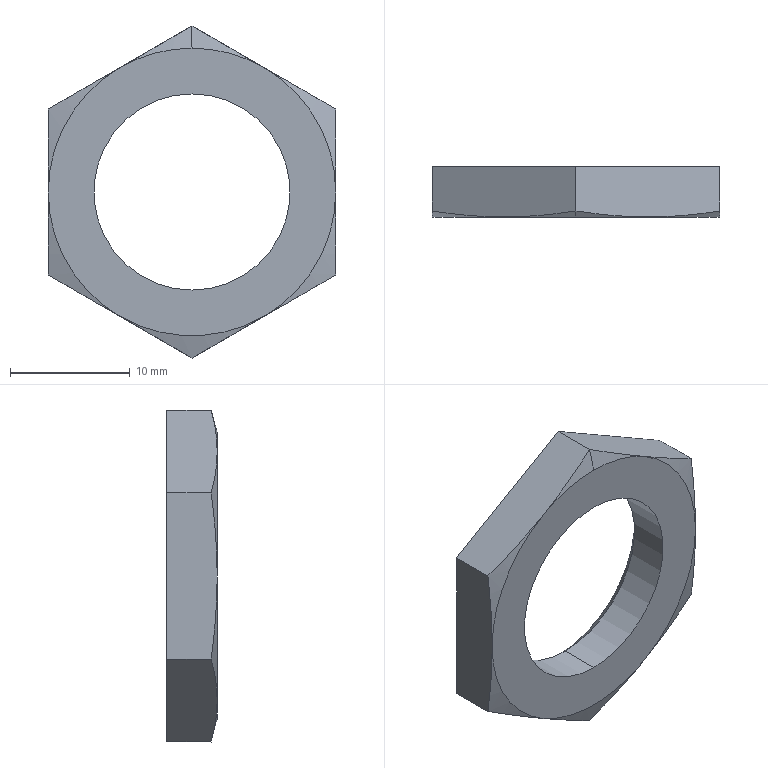Part | SolidWorks | features BaseBody 1 | 1 solid | 19 faces | box 24 x 4.2 x 27.713 mm | volume 1186 mm3 | cone 9 | plane 8 | cylinder 2 | commonest cylinder face diameters 16.376 x2
STEP:
#1=CARTESIAN_POINT('',(137.047,1614.26,-1167.188));
#2=VERTEX_POINT('',#1);
#3=CARTESIAN_POINT('',(137.047,1614.26,-1150.812));
#4=VERTEX_POINT('',#3);
#5=CARTESIAN_POINT('',(137.047,1614.26,-1159.));
#6=DIRECTION('',(0.,1.,0.));
#7=DIRECTION('',(0.,0.,-1.));
#8=AXIS2_PLACEMENT_3D('',#5,#6,#7);
#9=CIRCLE('',#8,8.188);
#10=EDGE_CURVE('',#2,#4,#9,.T.);
#11=ORIENTED_EDGE('',*,*,#10,.F.);
#12=CARTESIAN_POINT('',(137.047,1615.079,-1168.007));
#13=VERTEX_POINT('',#12);
#14=CARTESIAN_POINT('',(137.047,1615.079,-1168.007));
#15=DIRECTION('',(0.,0.7071,-0.7071));
#16=VECTOR('',#15,1000.);
#17=LINE('',#14,#16);
#18=EDGE_CURVE('',#2,#13,#17,.T.);
#19=ORIENTED_EDGE('',*,*,#18,.T.);
#20=CARTESIAN_POINT('',(137.047,1615.079,-1149.993));
#21=VERTEX_POINT('',#20);
#22=CARTESIAN_POINT('',(137.047,1615.079,-1159.));
#23=DIRECTION('',(0.,-1.,0.));
#24=DIRECTION('',(0.,0.,1.));
#25=AXIS2_PLACEMENT_3D('',#22,#23,#24);
#26=CIRCLE('',#25,9.007);
#27=EDGE_CURVE('',#21,#13,#26,.T.);
#28=ORIENTED_EDGE('',*,*,#27,.F.);
#29=CARTESIAN_POINT('',(137.047,1615.079,-1149.993));
#30=DIRECTION('',(0.,0.7071,0.7071));
#31=VECTOR('',#30,1000.);
#32=LINE('',#29,#31);
#33=EDGE_CURVE('',#4,#21,#32,.T.);
#34=ORIENTED_EDGE('',*,*,#33,.F.);
#35=EDGE_LOOP('',(#11,#19,#28,#34));
#36=FACE_OUTER_BOUND('',#35,.T.);
#37=CARTESIAN_POINT('',(137.047,1615.079,-1159.));
#38=DIRECTION('',(0.,1.,0.));
#39=DIRECTION('',(0.,0.,1.));
#40=AXIS2_PLACEMENT_3D('',#37,#38,#39);
#41=CONICAL_SURFACE('',#40,9.007,0.7854);
#42=ADVANCED_FACE('',(#36),#41,.F.);
#43=CARTESIAN_POINT('',(137.047,1610.879,-1167.188));
#44=VERTEX_POINT('',#43);
#45=CARTESIAN_POINT('',(137.047,1610.879,-1150.812));
#46=VERTEX_POINT('',#45);
#47=CARTESIAN_POINT('',(137.047,1610.879,-1159.));
#48=DIRECTION('',(0.,1.,0.));
#49=DIRECTION('',(0.,0.,1.));
#50=AXIS2_PLACEMENT_3D('',#47,#48,#49);
#51=CIRCLE('',#50,8.188);
#52=EDGE_CURVE('',#44,#46,#51,.T.);
#53=ORIENTED_EDGE('',*,*,#52,.F.);
#54=CARTESIAN_POINT('',(137.047,1610.879,-1167.188));
#55=DIRECTION('',(0.,1.,0.));
#56=VECTOR('',#55,1000.);
#57=LINE('',#54,#56);
#58=EDGE_CURVE('',#44,#2,#57,.T.);
#59=ORIENTED_EDGE('',*,*,#58,.T.);
#60=ORIENTED_EDGE('',*,*,#10,.T.);
#61=CARTESIAN_POINT('',(137.047,1610.879,-1150.812));
#62=DIRECTION('',(0.,1.,0.));
#63=VECTOR('',#62,1000.);
#64=LINE('',#61,#63);
#65=EDGE_CURVE('',#46,#4,#64,.T.);
#66=ORIENTED_EDGE('',*,*,#65,.F.);
#67=EDGE_LOOP('',(#53,#59,#60,#66));
#68=FACE_OUTER_BOUND('',#67,.T.);
#69=CARTESIAN_POINT('',(137.047,1610.879,-1159.));
#70=DIRECTION('',(0.,1.,0.));
#71=DIRECTION('',(0.,0.,1.));
#72=AXIS2_PLACEMENT_3D('',#69,#70,#71);
#73=CYLINDRICAL_SURFACE('',#72,8.188);
#74=ADVANCED_FACE('',(#68),#73,.F.);
#75=CARTESIAN_POINT('',(131.047,1610.879,-1148.608));
#76=VERTEX_POINT('',#75);
#77=CARTESIAN_POINT('',(137.047,1610.879,-1147.));
#78=VERTEX_POINT('',#77);
#79=CARTESIAN_POINT('',(137.047,1610.879,-1159.));
#80=DIRECTION('',(0.,1.,0.));
#81=DIRECTION('',(0.,0.,1.));
#82=AXIS2_PLACEMENT_3D('',#79,#80,#81);
#83=CIRCLE('',#82,12.);
#84=EDGE_CURVE('',#76,#78,#83,.T.);
#85=ORIENTED_EDGE('',*,*,#84,.T.);
#86=CARTESIAN_POINT('',(137.047,1611.376,-1145.144));
#87=VERTEX_POINT('',#86);
#88=CARTESIAN_POINT('',(137.047,1611.379,-1145.132));
#89=DIRECTION('',(0.,0.2588,0.9659));
#90=VECTOR('',#89,1000.);
#91=LINE('',#88,#90);
#92=EDGE_CURVE('',#78,#87,#91,.T.);
#93=ORIENTED_EDGE('',*,*,#92,.T.);
#94=CARTESIAN_POINT('',(131.047,1610.879,-1148.608));
#95=CARTESIAN_POINT('',(132.052,1610.879,-1148.027));
#96=CARTESIAN_POINT('',(133.054,1610.925,-1147.449));
#97=CARTESIAN_POINT('',(135.054,1611.097,-1146.294));
#98=CARTESIAN_POINT('',(136.051,1611.222,-1145.718));
#99=CARTESIAN_POINT('',(137.047,1611.376,-1145.144));
#100=B_SPLINE_CURVE_WITH_KNOTS('',3,(#94,#95,#96,#97,#98,#99),.UNSPECIFIED.,.F.,.F.,(4,2,4),(0.,0.003473,0.006946),.UNSPECIFIED.);
#101=EDGE_CURVE('',#76,#87,#100,.T.);
#102=ORIENTED_EDGE('',*,*,#101,.F.);
#103=EDGE_LOOP('',(#85,#93,#102));
#104=FACE_OUTER_BOUND('',#103,.T.);
#105=CARTESIAN_POINT('',(137.047,1611.379,-1159.));
#106=DIRECTION('',(0.,1.,0.));
#107=DIRECTION('',(0.,0.,1.));
#108=AXIS2_PLACEMENT_3D('',#105,#106,#107);
#109=CONICAL_SURFACE('',#108,13.868,1.309);
#110=ADVANCED_FACE('',(#104),#109,.T.);
#111=ORIENTED_EDGE('',*,*,#27,.T.);
#112=CARTESIAN_POINT('',(137.047,1615.079,-1159.));
#113=DIRECTION('',(0.,-1.,0.));
#114=DIRECTION('',(0.,0.,1.));
#115=AXIS2_PLACEMENT_3D('',#112,#113,#114);
#116=CIRCLE('',#115,9.007);
#117=EDGE_CURVE('',#13,#21,#116,.T.);
#118=ORIENTED_EDGE('',*,*,#117,.T.);
#119=EDGE_LOOP('',(#111,#118));
#120=FACE_BOUND('',#119,.T.);
#121=CARTESIAN_POINT('',(137.047,1615.079,-1145.144));
#122=VERTEX_POINT('',#121);
#123=CARTESIAN_POINT('',(149.047,1615.079,-1152.072));
#124=VERTEX_POINT('',#123);
#125=CARTESIAN_POINT('',(137.047,1615.079,-1145.144));
#126=DIRECTION('',(0.866,0.,-0.5));
#127=VECTOR('',#126,1000.);
#128=LINE('',#125,#127);
#129=EDGE_CURVE('',#122,#124,#128,.T.);
#130=ORIENTED_EDGE('',*,*,#129,.T.);
#131=CARTESIAN_POINT('',(149.047,1615.079,-1165.928));
#132=VERTEX_POINT('',#131);
#133=CARTESIAN_POINT('',(149.047,1615.079,-1165.928));
#134=DIRECTION('',(0.,0.,-1.));
#135=VECTOR('',#134,1000.);
#136=LINE('',#133,#135);
#137=EDGE_CURVE('',#124,#132,#136,.T.);
#138=ORIENTED_EDGE('',*,*,#137,.T.);
#139=CARTESIAN_POINT('',(137.047,1615.079,-1172.856));
#140=VERTEX_POINT('',#139);
#141=CARTESIAN_POINT('',(149.047,1615.079,-1165.928));
#142=DIRECTION('',(-0.866,0.,-0.5));
#143=VECTOR('',#142,1000.);
#144=LINE('',#141,#143);
#145=EDGE_CURVE('',#132,#140,#144,.T.);
#146=ORIENTED_EDGE('',*,*,#145,.T.);
#147=CARTESIAN_POINT('',(125.047,1615.079,-1165.928));
#148=VERTEX_POINT('',#147);
#149=CARTESIAN_POINT('',(137.047,1615.079,-1172.856));
#150=DIRECTION('',(-0.866,0.,0.5));
#151=VECTOR('',#150,1000.);
#152=LINE('',#149,#151);
#153=EDGE_CURVE('',#140,#148,#152,.T.);
#154=ORIENTED_EDGE('',*,*,#153,.T.);
#155=CARTESIAN_POINT('',(125.047,1615.079,-1152.072));
#156=VERTEX_POINT('',#155);
#157=CARTESIAN_POINT('',(125.047,1615.079,-1165.928));
#158=DIRECTION('',(0.,0.,1.));
#159=VECTOR('',#158,1000.);
#160=LINE('',#157,#159);
#161=EDGE_CURVE('',#148,#156,#160,.T.);
#162=ORIENTED_EDGE('',*,*,#161,.T.);
#163=CARTESIAN_POINT('',(125.047,1615.079,-1152.072));
#164=DIRECTION('',(0.866,0.,0.5));
#165=VECTOR('',#164,1000.);
#166=LINE('',#163,#165);
#167=EDGE_CURVE('',#156,#122,#166,.T.);
#168=ORIENTED_EDGE('',*,*,#167,.T.);
#169=EDGE_LOOP('',(#130,#138,#146,#154,#162,#168));
#170=FACE_OUTER_BOUND('',#169,.T.);
#171=CARTESIAN_POINT('',(149.047,1615.079,-1165.928));
#172=DIRECTION('',(0.,1.,0.));
#173=DIRECTION('',(0.,0.,1.));
#174=AXIS2_PLACEMENT_3D('',#171,#172,#173);
#175=PLANE('',#174);
#176=ADVANCED_FACE('',(#120,#170),#175,.T.);
#177=ORIENTED_EDGE('',*,*,#18,.F.);
#178=CARTESIAN_POINT('',(137.047,1614.26,-1159.));
#179=DIRECTION('',(0.,1.,0.));
#180=DIRECTION('',(0.,0.,-1.));
#181=AXIS2_PLACEMENT_3D('',#178,#179,#180);
#182=CIRCLE('',#181,8.188);
#183=EDGE_CURVE('',#4,#2,#182,.T.);
#184=ORIENTED_EDGE('',*,*,#183,.F.);
#185=ORIENTED_EDGE('',*,*,#33,.T.);
#186=ORIENTED_EDGE('',*,*,#117,.F.);
#187=EDGE_LOOP('',(#177,#184,#185,#186));
#188=FACE_OUTER_BOUND('',#187,.T.);
#189=CARTESIAN_POINT('',(137.047,1615.079,-1159.));
#190=DIRECTION('',(0.,1.,0.));
#191=DIRECTION('',(0.,0.,1.));
#192=AXIS2_PLACEMENT_3D('',#189,#190,#191);
#193=CONICAL_SURFACE('',#192,9.007,0.7854);
#194=ADVANCED_FACE('',(#188),#193,.F.);
#195=CARTESIAN_POINT('',(149.047,1611.376,-1152.072));
#196=VERTEX_POINT('',#195);
#197=CARTESIAN_POINT('',(149.047,1610.879,-1159.));
#198=VERTEX_POINT('',#197);
#199=CARTESIAN_POINT('',(149.047,1611.376,-1152.072));
#200=CARTESIAN_POINT('',(149.047,1611.222,-1153.221));
#201=CARTESIAN_POINT('',(149.047,1611.097,-1154.373));
#202=CARTESIAN_POINT('',(149.047,1610.925,-1156.682));
#203=CARTESIAN_POINT('',(149.047,1610.879,-1157.839));
#204=CARTESIAN_POINT('',(149.047,1610.879,-1159.));
#205=B_SPLINE_CURVE_WITH_KNOTS('',3,(#199,#200,#201,#202,#203,#204),.UNSPECIFIED.,.F.,.F.,(4,2,4),(0.,0.003473,0.006946),.UNSPECIFIED.);
#206=EDGE_CURVE('',#196,#198,#205,.T.);
#207=ORIENTED_EDGE('',*,*,#206,.T.);
#208=CARTESIAN_POINT('',(149.047,1611.376,-1165.928));
#209=VERTEX_POINT('',#208);
#210=CARTESIAN_POINT('',(149.047,1610.879,-1159.));
#211=CARTESIAN_POINT('',(149.047,1610.879,-1160.161));
#212=CARTESIAN_POINT('',(149.047,1610.925,-1161.318));
#213=CARTESIAN_POINT('',(149.047,1611.097,-1163.627));
#214=CARTESIAN_POINT('',(149.047,1611.222,-1164.779));
#215=CARTESIAN_POINT('',(149.047,1611.376,-1165.928));
#216=B_SPLINE_CURVE_WITH_KNOTS('',3,(#210,#211,#212,#213,#214,#215),.UNSPECIFIED.,.F.,.F.,(4,2,4),(0.,0.003473,0.006946),.UNSPECIFIED.);
#217=EDGE_CURVE('',#198,#209,#216,.T.);
#218=ORIENTED_EDGE('',*,*,#217,.T.);
#219=CARTESIAN_POINT('',(149.047,1610.879,-1165.928));
#220=DIRECTION('',(0.,1.,0.));
#221=VECTOR('',#220,1000.);
#222=LINE('',#219,#221);
#223=EDGE_CURVE('',#209,#132,#222,.T.);
#224=ORIENTED_EDGE('',*,*,#223,.T.);
#225=ORIENTED_EDGE('',*,*,#137,.F.);
#226=CARTESIAN_POINT('',(149.047,1610.879,-1152.072));
#227=DIRECTION('',(0.,-1.,0.));
#228=VECTOR('',#227,1000.);
#229=LINE('',#226,#228);
#230=EDGE_CURVE('',#124,#196,#229,.T.);
#231=ORIENTED_EDGE('',*,*,#230,.T.);
#232=EDGE_LOOP('',(#207,#218,#224,#225,#231));
#233=FACE_OUTER_BOUND('',#232,.T.);
#234=CARTESIAN_POINT('',(149.047,1610.879,-1152.072));
#235=DIRECTION('',(1.,0.,0.));
#236=DIRECTION('',(0.,0.,-1.));
#237=AXIS2_PLACEMENT_3D('',#234,#235,#236);
#238=PLANE('',#237);
#239=ADVANCED_FACE('',(#233),#238,.T.);
#240=CARTESIAN_POINT('',(143.047,1610.879,-1148.608));
#241=VERTEX_POINT('',#240);
#242=CARTESIAN_POINT('',(137.047,1611.376,-1145.144));
#243=CARTESIAN_POINT('',(138.042,1611.222,-1145.718));
#244=CARTESIAN_POINT('',(139.039,1611.097,-1146.294));
#245=CARTESIAN_POINT('',(141.039,1610.925,-1147.449));
#246=CARTESIAN_POINT('',(142.041,1610.879,-1148.027));
#247=CARTESIAN_POINT('',(143.047,1610.879,-1148.608));
#248=B_SPLINE_CURVE_WITH_KNOTS('',3,(#242,#243,#244,#245,#246,#247),.UNSPECIFIED.,.F.,.F.,(4,2,4),(0.,0.003473,0.006946),.UNSPECIFIED.);
#249=EDGE_CURVE('',#87,#241,#248,.T.);
#250=ORIENTED_EDGE('',*,*,#249,.T.);
#251=CARTESIAN_POINT('',(143.047,1610.879,-1148.608));
#252=CARTESIAN_POINT('',(144.052,1610.879,-1149.188));
#253=CARTESIAN_POINT('',(145.054,1610.925,-1149.767));
#254=CARTESIAN_POINT('',(147.054,1611.097,-1150.921));
#255=CARTESIAN_POINT('',(148.051,1611.222,-1151.497));
#256=CARTESIAN_POINT('',(149.047,1611.376,-1152.072));
#257=B_SPLINE_CURVE_WITH_KNOTS('',3,(#251,#252,#253,#254,#255,#256),.UNSPECIFIED.,.F.,.F.,(4,2,4),(0.,0.003473,0.006946),.UNSPECIFIED.);
#258=EDGE_CURVE('',#241,#196,#257,.T.);
#259=ORIENTED_EDGE('',*,*,#258,.T.);
#260=ORIENTED_EDGE('',*,*,#230,.F.);
#261=ORIENTED_EDGE('',*,*,#129,.F.);
#262=CARTESIAN_POINT('',(137.047,1610.879,-1145.144));
#263=DIRECTION('',(0.,-1.,0.));
#264=VECTOR('',#263,1000.);
#265=LINE('',#262,#264);
#266=EDGE_CURVE('',#122,#87,#265,.T.);
#267=ORIENTED_EDGE('',*,*,#266,.T.);
#268=EDGE_LOOP('',(#250,#259,#260,#261,#267));
#269=FACE_OUTER_BOUND('',#268,.T.);
#270=CARTESIAN_POINT('',(137.047,1610.879,-1145.144));
#271=DIRECTION('',(0.5,0.,0.866));
#272=DIRECTION('',(0.866,0.,-0.5));
#273=AXIS2_PLACEMENT_3D('',#270,#271,#272);
#274=PLANE('',#273);
#275=ADVANCED_FACE('',(#269),#274,.T.);
#276=CARTESIAN_POINT('',(125.047,1611.376,-1152.072));
#277=VERTEX_POINT('',#276);
#278=CARTESIAN_POINT('',(125.047,1611.376,-1152.072));
#279=CARTESIAN_POINT('',(126.042,1611.222,-1151.497));
#280=CARTESIAN_POINT('',(127.039,1611.097,-1150.921));
#281=CARTESIAN_POINT('',(129.039,1610.925,-1149.767));
#282=CARTESIAN_POINT('',(130.041,1610.879,-1149.188));
#283=CARTESIAN_POINT('',(131.047,1610.879,-1148.608));
#284=B_SPLINE_CURVE_WITH_KNOTS('',3,(#278,#279,#280,#281,#282,#283),.UNSPECIFIED.,.F.,.F.,(4,2,4),(0.,0.003473,0.006946),.UNSPECIFIED.);
#285=EDGE_CURVE('',#277,#76,#284,.T.);
#286=ORIENTED_EDGE('',*,*,#285,.T.);
#287=ORIENTED_EDGE('',*,*,#101,.T.);
#288=ORIENTED_EDGE('',*,*,#266,.F.);
#289=ORIENTED_EDGE('',*,*,#167,.F.);
#290=CARTESIAN_POINT('',(125.047,1610.879,-1152.072));
#291=DIRECTION('',(0.,-1.,0.));
#292=VECTOR('',#291,1000.);
#293=LINE('',#290,#292);
#294=EDGE_CURVE('',#156,#277,#293,.T.);
#295=ORIENTED_EDGE('',*,*,#294,.T.);
#296=EDGE_LOOP('',(#286,#287,#288,#289,#295));
#297=FACE_OUTER_BOUND('',#296,.T.);
#298=CARTESIAN_POINT('',(125.047,1610.879,-1152.072));
#299=DIRECTION('',(-0.5,0.,0.866));
#300=DIRECTION('',(0.866,0.,0.5));
#301=AXIS2_PLACEMENT_3D('',#298,#299,#300);
#302=PLANE('',#301);
#303=ADVANCED_FACE('',(#297),#302,.T.);
#304=CARTESIAN_POINT('',(125.047,1611.376,-1165.928));
#305=VERTEX_POINT('',#304);
#306=CARTESIAN_POINT('',(125.047,1610.879,-1159.));
#307=VERTEX_POINT('',#306);
#308=CARTESIAN_POINT('',(125.047,1611.376,-1165.928));
#309=CARTESIAN_POINT('',(125.047,1611.222,-1164.779));
#310=CARTESIAN_POINT('',(125.047,1611.097,-1163.627));
#311=CARTESIAN_POINT('',(125.047,1610.925,-1161.318));
#312=CARTESIAN_POINT('',(125.047,1610.879,-1160.161));
#313=CARTESIAN_POINT('',(125.047,1610.879,-1159.));
#314=B_SPLINE_CURVE_WITH_KNOTS('',3,(#308,#309,#310,#311,#312,#313),.UNSPECIFIED.,.F.,.F.,(4,2,4),(0.,0.003473,0.006946),.UNSPECIFIED.);
#315=EDGE_CURVE('',#305,#307,#314,.T.);
#316=ORIENTED_EDGE('',*,*,#315,.T.);
#317=CARTESIAN_POINT('',(125.047,1610.879,-1159.));
#318=CARTESIAN_POINT('',(125.047,1610.879,-1157.839));
#319=CARTESIAN_POINT('',(125.047,1610.925,-1156.682));
#320=CARTESIAN_POINT('',(125.047,1611.097,-1154.373));
#321=CARTESIAN_POINT('',(125.047,1611.222,-1153.221));
#322=CARTESIAN_POINT('',(125.047,1611.376,-1152.072));
#323=B_SPLINE_CURVE_WITH_KNOTS('',3,(#317,#318,#319,#320,#321,#322),.UNSPECIFIED.,.F.,.F.,(4,2,4),(0.,0.003473,0.006946),.UNSPECIFIED.);
#324=EDGE_CURVE('',#307,#277,#323,.T.);
#325=ORIENTED_EDGE('',*,*,#324,.T.);
#326=ORIENTED_EDGE('',*,*,#294,.F.);
#327=ORIENTED_EDGE('',*,*,#161,.F.);
#328=CARTESIAN_POINT('',(125.047,1610.879,-1165.928));
#329=DIRECTION('',(0.,-1.,0.));
#330=VECTOR('',#329,1000.);
#331=LINE('',#328,#330);
#332=EDGE_CURVE('',#148,#305,#331,.T.);
#333=ORIENTED_EDGE('',*,*,#332,.T.);
#334=EDGE_LOOP('',(#316,#325,#326,#327,#333));
#335=FACE_OUTER_BOUND('',#334,.T.);
#336=CARTESIAN_POINT('',(125.047,1610.879,-1165.928));
#337=DIRECTION('',(-1.,0.,0.));
#338=DIRECTION('',(0.,0.,1.));
#339=AXIS2_PLACEMENT_3D('',#336,#337,#338);
#340=PLANE('',#339);
#341=ADVANCED_FACE('',(#335),#340,.T.);
#342=CARTESIAN_POINT('',(137.047,1611.376,-1172.856));
#343=VERTEX_POINT('',#342);
#344=CARTESIAN_POINT('',(131.047,1610.879,-1169.392));
#345=VERTEX_POINT('',#344);
#346=CARTESIAN_POINT('',(137.047,1611.376,-1172.856));
#347=CARTESIAN_POINT('',(136.051,1611.222,-1172.282));
#348=CARTESIAN_POINT('',(135.054,1611.097,-1171.706));
#349=CARTESIAN_POINT('',(133.054,1610.925,-1170.551));
#350=CARTESIAN_POINT('',(132.052,1610.879,-1169.973));
#351=CARTESIAN_POINT('',(131.047,1610.879,-1169.392));
#352=B_SPLINE_CURVE_WITH_KNOTS('',3,(#346,#347,#348,#349,#350,#351),.UNSPECIFIED.,.F.,.F.,(4,2,4),(0.,0.003473,0.006946),.UNSPECIFIED.);
#353=EDGE_CURVE('',#343,#345,#352,.T.);
#354=ORIENTED_EDGE('',*,*,#353,.T.);
#355=CARTESIAN_POINT('',(131.047,1610.879,-1169.392));
#356=CARTESIAN_POINT('',(130.041,1610.879,-1168.812));
#357=CARTESIAN_POINT('',(129.039,1610.925,-1168.233));
#358=CARTESIAN_POINT('',(127.039,1611.097,-1167.079));
#359=CARTESIAN_POINT('',(126.042,1611.222,-1166.503));
#360=CARTESIAN_POINT('',(125.047,1611.376,-1165.928));
#361=B_SPLINE_CURVE_WITH_KNOTS('',3,(#355,#356,#357,#358,#359,#360),.UNSPECIFIED.,.F.,.F.,(4,2,4),(0.,0.003473,0.006946),.UNSPECIFIED.);
#362=EDGE_CURVE('',#345,#305,#361,.T.);
#363=ORIENTED_EDGE('',*,*,#362,.T.);
#364=ORIENTED_EDGE('',*,*,#332,.F.);
#365=ORIENTED_EDGE('',*,*,#153,.F.);
#366=CARTESIAN_POINT('',(137.047,1610.879,-1172.856));
#367=DIRECTION('',(0.,-1.,0.));
#368=VECTOR('',#367,1000.);
#369=LINE('',#366,#368);
#370=EDGE_CURVE('',#140,#343,#369,.T.);
#371=ORIENTED_EDGE('',*,*,#370,.T.);
#372=EDGE_LOOP('',(#354,#363,#364,#365,#371));
#373=FACE_OUTER_BOUND('',#372,.T.);
#374=CARTESIAN_POINT('',(137.047,1610.879,-1172.856));
#375=DIRECTION('',(-0.5,0.,-0.866));
#376=DIRECTION('',(-0.866,0.,0.5));
#377=AXIS2_PLACEMENT_3D('',#374,#375,#376);
#378=PLANE('',#377);
#379=ADVANCED_FACE('',(#373),#378,.T.);
#380=CARTESIAN_POINT('',(143.047,1610.879,-1169.392));
#381=VERTEX_POINT('',#380);
#382=CARTESIAN_POINT('',(149.047,1611.376,-1165.928));
#383=CARTESIAN_POINT('',(148.051,1611.222,-1166.503));
#384=CARTESIAN_POINT('',(147.054,1611.097,-1167.079));
#385=CARTESIAN_POINT('',(145.054,1610.925,-1168.233));
#386=CARTESIAN_POINT('',(144.052,1610.879,-1168.812));
#387=CARTESIAN_POINT('',(143.047,1610.879,-1169.392));
#388=B_SPLINE_CURVE_WITH_KNOTS('',3,(#382,#383,#384,#385,#386,#387),.UNSPECIFIED.,.F.,.F.,(4,2,4),(0.,0.003473,0.006946),.UNSPECIFIED.);
#389=EDGE_CURVE('',#209,#381,#388,.T.);
#390=ORIENTED_EDGE('',*,*,#389,.T.);
#391=CARTESIAN_POINT('',(143.047,1610.879,-1169.392));
#392=CARTESIAN_POINT('',(142.041,1610.879,-1169.973));
#393=CARTESIAN_POINT('',(141.039,1610.925,-1170.551));
#394=CARTESIAN_POINT('',(139.039,1611.097,-1171.706));
#395=CARTESIAN_POINT('',(138.042,1611.222,-1172.282));
#396=CARTESIAN_POINT('',(137.047,1611.376,-1172.856));
#397=B_SPLINE_CURVE_WITH_KNOTS('',3,(#391,#392,#393,#394,#395,#396),.UNSPECIFIED.,.F.,.F.,(4,2,4),(0.,0.003473,0.006946),.UNSPECIFIED.);
#398=EDGE_CURVE('',#381,#343,#397,.T.);
#399=ORIENTED_EDGE('',*,*,#398,.T.);
#400=ORIENTED_EDGE('',*,*,#370,.F.);
#401=ORIENTED_EDGE('',*,*,#145,.F.);
#402=ORIENTED_EDGE('',*,*,#223,.F.);
#403=EDGE_LOOP('',(#390,#399,#400,#401,#402));
#404=FACE_OUTER_BOUND('',#403,.T.);
#405=CARTESIAN_POINT('',(149.047,1610.879,-1165.928));
#406=DIRECTION('',(0.5,0.,-0.866));
#407=DIRECTION('',(-0.866,0.,-0.5));
#408=AXIS2_PLACEMENT_3D('',#405,#406,#407);
#409=PLANE('',#408);
#410=ADVANCED_FACE('',(#404),#409,.T.);
#411=ORIENTED_EDGE('',*,*,#58,.F.);
#412=CARTESIAN_POINT('',(137.047,1610.879,-1159.));
#413=DIRECTION('',(0.,1.,0.));
#414=DIRECTION('',(0.,0.,1.));
#415=AXIS2_PLACEMENT_3D('',#412,#413,#414);
#416=CIRCLE('',#415,8.188);
#417=EDGE_CURVE('',#46,#44,#416,.T.);
#418=ORIENTED_EDGE('',*,*,#417,.F.);
#419=ORIENTED_EDGE('',*,*,#65,.T.);
#420=ORIENTED_EDGE('',*,*,#183,.T.);
#421=EDGE_LOOP('',(#411,#418,#419,#420));
#422=FACE_OUTER_BOUND('',#421,.T.);
#423=CARTESIAN_POINT('',(137.047,1610.879,-1159.));
#424=DIRECTION('',(0.,1.,0.));
#425=DIRECTION('',(0.,0.,1.));
#426=AXIS2_PLACEMENT_3D('',#423,#424,#425);
#427=CYLINDRICAL_SURFACE('',#426,8.188);
#428=ADVANCED_FACE('',(#422),#427,.F.);
#429=ORIENTED_EDGE('',*,*,#389,.F.);
#430=ORIENTED_EDGE('',*,*,#217,.F.);
#431=CARTESIAN_POINT('',(137.047,1610.879,-1159.));
#432=DIRECTION('',(0.,1.,0.));
#433=DIRECTION('',(-1.,0.,0.));
#434=AXIS2_PLACEMENT_3D('',#431,#432,#433);
#435=CIRCLE('',#434,12.);
#436=EDGE_CURVE('',#198,#381,#435,.T.);
#437=ORIENTED_EDGE('',*,*,#436,.T.);
#438=EDGE_LOOP('',(#429,#430,#437));
#439=FACE_OUTER_BOUND('',#438,.T.);
#440=CARTESIAN_POINT('',(137.047,1611.379,-1159.));
#441=DIRECTION('',(0.,1.,0.));
#442=DIRECTION('',(-1.,0.,0.));
#443=AXIS2_PLACEMENT_3D('',#440,#441,#442);
#444=CONICAL_SURFACE('',#443,13.868,1.309);
#445=ADVANCED_FACE('',(#439),#444,.T.);
#446=CARTESIAN_POINT('',(137.047,1610.879,-1159.));
#447=DIRECTION('',(0.,1.,0.));
#448=DIRECTION('',(0.,0.,1.));
#449=AXIS2_PLACEMENT_3D('',#446,#447,#448);
#450=CIRCLE('',#449,12.);
#451=EDGE_CURVE('',#241,#198,#450,.T.);
#452=ORIENTED_EDGE('',*,*,#451,.T.);
#453=ORIENTED_EDGE('',*,*,#206,.F.);
#454=ORIENTED_EDGE('',*,*,#258,.F.);
#455=EDGE_LOOP('',(#452,#453,#454));
#456=FACE_OUTER_BOUND('',#455,.T.);
#457=CARTESIAN_POINT('',(137.047,1611.379,-1159.));
#458=DIRECTION('',(0.,1.,0.));
#459=DIRECTION('',(0.,0.,1.));
#460=AXIS2_PLACEMENT_3D('',#457,#458,#459);
#461=CONICAL_SURFACE('',#460,13.868,1.309);
#462=ADVANCED_FACE('',(#456),#461,.T.);
#463=ORIENTED_EDGE('',*,*,#92,.F.);
#464=CARTESIAN_POINT('',(137.047,1610.879,-1159.));
#465=DIRECTION('',(0.,1.,0.));
#466=DIRECTION('',(0.,0.,1.));
#467=AXIS2_PLACEMENT_3D('',#464,#465,#466);
#468=CIRCLE('',#467,12.);
#469=EDGE_CURVE('',#78,#241,#468,.T.);
#470=ORIENTED_EDGE('',*,*,#469,.T.);
#471=ORIENTED_EDGE('',*,*,#249,.F.);
#472=EDGE_LOOP('',(#463,#470,#471));
#473=FACE_OUTER_BOUND('',#472,.T.);
#474=CARTESIAN_POINT('',(137.047,1611.379,-1159.));
#475=DIRECTION('',(0.,1.,0.));
#476=DIRECTION('',(0.,0.,1.));
#477=AXIS2_PLACEMENT_3D('',#474,#475,#476);
#478=CONICAL_SURFACE('',#477,13.868,1.309);
#479=ADVANCED_FACE('',(#473),#478,.T.);
#480=CARTESIAN_POINT('',(137.047,1610.879,-1159.));
#481=DIRECTION('',(0.,1.,0.));
#482=DIRECTION('',(0.,0.,1.));
#483=AXIS2_PLACEMENT_3D('',#480,#481,#482);
#484=CIRCLE('',#483,12.);
#485=EDGE_CURVE('',#307,#76,#484,.T.);
#486=ORIENTED_EDGE('',*,*,#485,.T.);
#487=ORIENTED_EDGE('',*,*,#285,.F.);
#488=ORIENTED_EDGE('',*,*,#324,.F.);
#489=EDGE_LOOP('',(#486,#487,#488));
#490=FACE_OUTER_BOUND('',#489,.T.);
#491=CARTESIAN_POINT('',(137.047,1611.379,-1159.));
#492=DIRECTION('',(0.,1.,0.));
#493=DIRECTION('',(0.,0.,1.));
#494=AXIS2_PLACEMENT_3D('',#491,#492,#493);
#495=CONICAL_SURFACE('',#494,13.868,1.309);
#496=ADVANCED_FACE('',(#490),#495,.T.);
#497=CARTESIAN_POINT('',(137.047,1610.879,-1159.));
#498=DIRECTION('',(0.,1.,0.));
#499=DIRECTION('',(-1.,0.,0.));
#500=AXIS2_PLACEMENT_3D('',#497,#498,#499);
#501=CIRCLE('',#500,12.);
#502=EDGE_CURVE('',#345,#307,#501,.T.);
#503=ORIENTED_EDGE('',*,*,#502,.T.);
#504=ORIENTED_EDGE('',*,*,#315,.F.);
#505=ORIENTED_EDGE('',*,*,#362,.F.);
#506=EDGE_LOOP('',(#503,#504,#505));
#507=FACE_OUTER_BOUND('',#506,.T.);
#508=CARTESIAN_POINT('',(137.047,1611.379,-1159.));
#509=DIRECTION('',(0.,1.,0.));
#510=DIRECTION('',(-1.,0.,0.));
#511=AXIS2_PLACEMENT_3D('',#508,#509,#510);
#512=CONICAL_SURFACE('',#511,13.868,1.309);
#513=ADVANCED_FACE('',(#507),#512,.T.);
#514=CARTESIAN_POINT('',(137.047,1610.879,-1159.));
#515=DIRECTION('',(0.,1.,0.));
#516=DIRECTION('',(0.,0.,1.));
#517=AXIS2_PLACEMENT_3D('',#514,#515,#516);
#518=CIRCLE('',#517,12.);
#519=EDGE_CURVE('',#381,#345,#518,.T.);
#520=ORIENTED_EDGE('',*,*,#519,.T.);
#521=ORIENTED_EDGE('',*,*,#353,.F.);
#522=ORIENTED_EDGE('',*,*,#398,.F.);
#523=EDGE_LOOP('',(#520,#521,#522));
#524=FACE_OUTER_BOUND('',#523,.T.);
#525=CARTESIAN_POINT('',(137.047,1611.379,-1159.));
#526=DIRECTION('',(0.,1.,0.));
#527=DIRECTION('',(0.,0.,1.));
#528=AXIS2_PLACEMENT_3D('',#525,#526,#527);
#529=CONICAL_SURFACE('',#528,13.868,1.309);
#530=ADVANCED_FACE('',(#524),#529,.T.);
#531=ORIENTED_EDGE('',*,*,#417,.T.);
#532=ORIENTED_EDGE('',*,*,#52,.T.);
#533=EDGE_LOOP('',(#531,#532));
#534=FACE_BOUND('',#533,.T.);
#535=ORIENTED_EDGE('',*,*,#451,.F.);
#536=ORIENTED_EDGE('',*,*,#469,.F.);
#537=ORIENTED_EDGE('',*,*,#84,.F.);
#538=ORIENTED_EDGE('',*,*,#485,.F.);
#539=ORIENTED_EDGE('',*,*,#502,.F.);
#540=ORIENTED_EDGE('',*,*,#519,.F.);
#541=ORIENTED_EDGE('',*,*,#436,.F.);
#542=EDGE_LOOP('',(#535,#536,#537,#538,#539,#540,#541));
#543=FACE_OUTER_BOUND('',#542,.T.);
#544=CARTESIAN_POINT('',(149.047,1610.879,-1165.928));
#545=DIRECTION('',(0.,1.,0.));
#546=DIRECTION('',(0.,0.,1.));
#547=AXIS2_PLACEMENT_3D('',#544,#545,#546);
#548=PLANE('',#547);
#549=ADVANCED_FACE('',(#534,#543),#548,.F.);
#550=CLOSED_SHELL('',(#42,#74,#110,#176,#194,#239,#275,#303,#341,#379,#410,#428,#445,#462,#479,#496,#513,#530,#549));
#551=MANIFOLD_SOLID_BREP('',#550);
#552=CARTESIAN_POINT('',(0.,0.,0.));
#553=DIRECTION('',(0.,0.,1.));
#554=DIRECTION('',(1.,0.,0.));
#555=AXIS2_PLACEMENT_3D('',#552,#553,#554);
#556=(LENGTH_UNIT()NAMED_UNIT(*)SI_UNIT(.MILLI.,.METRE.));
#557=UNCERTAINTY_MEASURE_WITH_UNIT(LENGTH_MEASURE(0.00001),#556,'','');
#558=(NAMED_UNIT(*)PLANE_ANGLE_UNIT()SI_UNIT($,.RADIAN.));
#559=(NAMED_UNIT(*)SI_UNIT($,.STERADIAN.)SOLID_ANGLE_UNIT());
#560=(GEOMETRIC_REPRESENTATION_CONTEXT(3)GLOBAL_UNCERTAINTY_ASSIGNED_CONTEXT((#557))GLOBAL_UNIT_ASSIGNED_CONTEXT((#556,#558,#559))REPRESENTATION_CONTEXT('',''));
#561=ADVANCED_BREP_SHAPE_REPRESENTATION('',(#551,#555),#560);